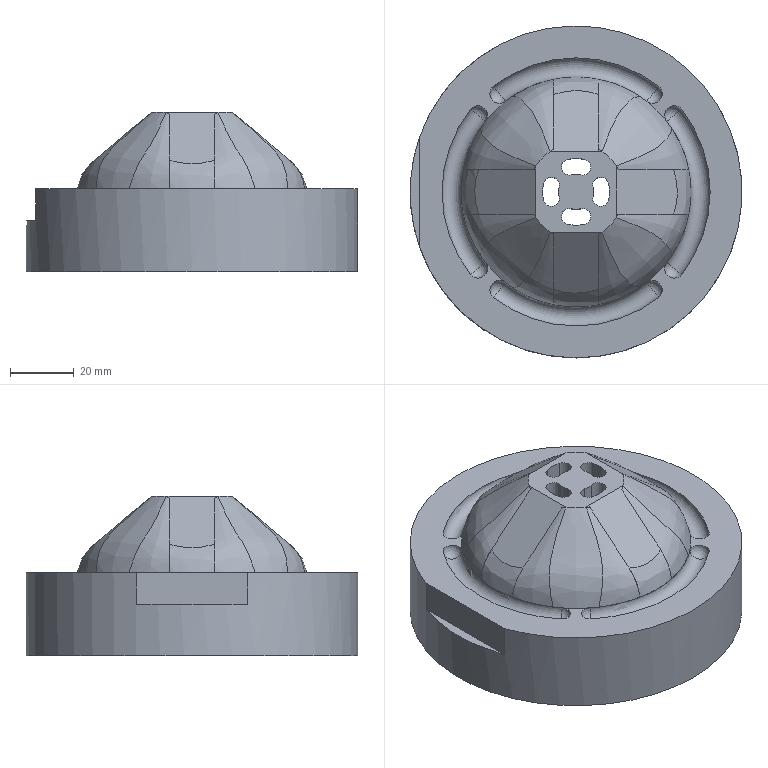NC program | NX | posted with a generic post | part box 104 x 104 x 49.86 mm
Lines 4139 to 5049 of 41131:
(ZLEVEL_PROFILE , TOOL : B12)
N8258 M6
N8260 G54
N8262 G17 G0 G90 X-5.745 Y-14.748 S3000 M3
N8264 G43 Z20. H0
N8266 Z0.2
N8268 G94 G1 X-6.948 Z0.168 F2000.
N8270 X-8.842 Y-14.619 Z0.119
N8272 X-9.264 Y-14.407 Z0.106
N8274 X-10.132 Y-13.832 Z0.079
N8276 X-12.11 Y-12.117 Z0.011
N8278 X-13.819 Y-10.134 Z-0.058
N8280 X-14.392 Y-9.264 Z-0.085
N8282 X-14.748 Y-8.085 Z-0.117
N8284 Y-1.181 Z-0.298
N8286 Y6.955 F2500.
N8288 X-14.7 Y6.986
N8290 X-14.632 Y8.788
N8292 X-14.619 Y8.842
N8294 G2 X-10.106 Y13.782 R13.681
N8296 G1 X-9.584 Y14.169
N8298 G2 X-8.085 Y14.748 R3.009
N8300 G1 X8.085
N8302 G2 X9.419 Y14.301 R2.214
N8304 G1 X10.506 Y13.48
N8306 G2 X14.182 Y9.513 R15.361
N8308 X14.748 Y8.085 R3.997
N8310 G1 Y-8.085
N8312 G2 X14.301 Y-9.419 R2.214
N8314 G1 X13.48 Y-10.506
N8316 G2 X9.513 Y-14.182 R15.361
N8318 X8.09 Y-14.748 R4.007
N8320 G1 X-6.948
N8322 X-8.842 Y-14.619
N8324 X-9.264 Y-14.407
N8326 G2 X-14.392 Y-9.264 R18.072
N8328 G1 X-14.748 Y-8.085
N8330 Y-1.181
N8332 X-15.113 Z-0.447
N8334 X-15.424 Z-0.597
N8336 Y-8.085
N8338 X-15.174 Y-9.264
N8340 G3 X-9.376 Y-15.111 R17.587
N8342 X-8.392 Y-15.39 R1.871
N8344 G1 X-6.983
N8346 X-6.953 Y-15.424
N8348 X8.09
N8350 X9.264 Y-15.174
N8352 G3 X15.062 Y-9.454 R17.608
N8354 X15.424 Y-8.194 R2.377
N8356 G1 Y8.087
N8358 X15.174 Y9.264
N8360 G3 X9.454 Y15.062 R17.608
N8362 X8.194 Y15.424 R2.377
N8364 G1 X-8.085
N8366 X-9.264 Y15.174
N8368 G3 X-14.097 Y10.803 R16.688
N8370 G1 X-14.907 Y9.713
N8372 G3 X-15.375 Y8.421 R2.263
N8374 G1 X-15.39 Y6.983
N8376 X-15.424 Y6.953
N8378 Y-1.181
N8380 X-15.696 Z-0.746
N8382 X-15.939 Z-0.895
N8384 Y6.951
N8386 X-15.855 Y8.85
N8388 X-15.733 Y9.264
N8390 G2 X-9.826 Y15.439 R17.411
N8392 X-8.088 Y15.939 R3.274
N8394 G1 X8.013
N8396 G2 X9.959 Y15.359 R3.557
N8398 X15.262 Y10.106 R18.618
N8400 X15.939 Y8.09 R3.89
N8402 G1 Y-8.013
N8404 G2 X15.359 Y-9.959 R3.557
N8406 X10.106 Y-15.262 R18.618
N8408 X8.09 Y-15.939 R3.891
N8410 G1 X-7.
N8412 X-8.85 Y-15.855
N8414 X-9.264 Y-15.733
N8416 G2 X-15.439 Y-9.826 R17.411
N8418 X-15.939 Y-8.088 R3.274
N8420 G1 Y-1.181
N8422 X-16.158 Z-1.044
N8424 X-16.359 Z-1.193
N8426 Y-8.1
N8428 G3 X-15.766 Y-10.106 R3.673
N8430 X-9.663 Y-16.001 R17.956
N8432 X-7. Y-16.359 R5.641
N8434 G1 X8.
N8436 G3 X10.106 Y-15.766 R3.809
N8438 X15.766 Y-10.106 R18.763
N8440 X16.359 Y-8.094 R3.673
N8442 G1 Y8.
N8444 G3 X15.766 Y10.106 R3.809
N8446 X10.106 Y15.766 R18.763
N8448 X8.094 Y16.359 R3.673
N8450 G1 X-8.16
N8452 G3 X-10.052 Y15.805 R3.507
N8454 X-15.159 Y11.001 R19.049
N8456 G1 X-15.583 Y10.419
N8458 G3 X-16.342 Y8.051 R3.95
N8460 G1 X-16.331 Y6.983
N8462 X-16.359 Y6.953
N8464 Y-1.181
N8466 X-16.544 Z-1.342
N8468 X-16.722 Z-1.491
N8470 Y8.301
N8472 G2 X-16.08 Y10.384 R3.7
N8474 X-15.159 Y11.651 R25.733
N8476 X-10.177 Y16.197 R19.698
N8478 X-8.377 Y16.722 R3.347
N8480 G1 X7.629
N8482 G2 X10.262 Y16.142 R3.863
N8484 X16.211 Y10.156 R19.742
N8486 X16.722 Y8.399 R3.271
N8488 G1 Y-7.629
N8490 G2 X16.142 Y-10.262 R3.863
N8492 X10.156 Y-16.211 R19.738
N8494 X8.399 Y-16.722 R3.271
N8496 G1 X-7.83
N8498 G2 X-10.187 Y-16.191 R3.553
N8500 X-16.21 Y-10.157 R19.734
N8502 X-16.722 Y-8.398 R3.277
N8504 G1 Y-1.181
N8506 X-17.078 Z-1.79
N8508 Y-7.086
N8510 X-17.079 Y-7.153
N8512 X-17.096 Y-7.579
N8514 X-17.11 Y-8.422
N8516 G3 X-16.695 Y-10.106 R4.099
N8518 X-10.106 Y-16.695 R20.371
N8520 X-7.089 Y-17.078 R5.61
N8522 G1 X7.086
N8524 X7.153 Y-17.079
N8526 X7.579 Y-17.096
N8528 X8.421 Y-17.11
N8530 G3 X10.106 Y-16.695 R4.115
N8532 X16.695 Y-10.106 R20.423
N8534 X17.078 Y-7.089 R5.61
N8536 G1 Y7.097
N8538 X17.08 Y7.136
N8540 X17.096 Y7.579
N8542 X17.11 Y8.421
N8544 G3 X16.695 Y10.106 R4.115
N8546 X10.106 Y16.695 R20.423
N8548 X7.089 Y17.078 R5.554
N8550 G1 X-7.097
N8552 X-7.171 Y17.079
N8554 X-7.579 Y17.096
N8556 X-8.422 Y17.11
N8558 G3 X-10.106 Y16.695 R4.099
N8560 X-16.418 Y10.586 R20.977
N8562 X-17.109 Y8.421 R4.089
N8564 G1 X-17.098 Y7.579
N8566 X-17.079 Y7.1
N8568 X-17.078 Y7.
N8570 Y-1.181
N8572 X-17.433 Z-2.088
N8574 Y6.8
N8576 X-17.493 Y8.05
N8578 G2 X-17.129 Y10.106 R4.7
N8580 X-10.245 Y17.044 R20.39
N8582 X-8.381 Y17.515 R3.25
N8584 G1 X-6.849 Y17.433
N8586 X6.876
N8588 X7.5 Y17.493
N8590 G2 X10.106 Y17.129 R5.65
N8592 X17.01 Y10.302 R20.395
N8594 X17.511 Y8.339 R3.419
N8596 G1 X17.433 Y6.815
N8598 Y-6.876
N8600 X17.488 Y-7.449
N8602 G2 X17.129 Y-10.106 R5.868
N8604 X10.312 Y-17.004 R20.387
N8606 X8.323 Y-17.511 R3.455
N8608 G1 X6.831 Y-17.433
N8610 X-6.876
N8612 X-7.449 Y-17.488
N8614 G2 X-10.106 Y-17.129 R5.868
N8616 X-17.04 Y-10.253 R20.382
N8618 X-17.514 Y-8.381 R3.268
N8620 G1 X-17.433 Y-6.831
N8622 Y-1.181
N8624 X-17.788 Z-2.386
N8626 Y-6.701
N8628 G3 X-17.553 Y-10.106 R7.601
N8630 X-10.106 Y-17.553 R20.25
N8632 X-7.824 Y-17.864 R5.669
N8634 G1 X-6.724 Y-17.788
N8636 X6.71
N8638 G3 X10.106 Y-17.553 R7.573
N8640 X17.553 Y-10.106 R20.25
N8642 X17.864 Y-7.824 R5.669
N8644 G1 X17.788 Y-6.724
N8646 Y6.71
N8648 G3 X17.553 Y10.106 R7.573
N8650 X10.106 Y17.553 R20.249
N8652 X7.824 Y17.864 R5.67
N8654 G1 X6.724 Y17.788
N8656 X-6.71
N8658 G3 X-10.106 Y17.553 R7.573
N8660 X-17.553 Y10.106 R20.25
N8662 X-17.864 Y7.824 R5.669
N8664 G1 X-17.788 Y6.724
N8666 Y-1.181
N8668 X-18.144 Z-2.684
N8670 Y6.672
N8672 X-18.224 Y7.539
N8674 G2 X-17.966 Y10.106 R6.747
N8676 X-17.02 Y11.696 R7.82
N8678 G1 X-16.563 Y12.29
N8680 G2 X-10.932 Y17.54 R23.494
N8682 X-9.06 Y18.194 R4.005
N8684 X-6.687 Y18.144 R11.148
N8686 G1 X6.688
N8688 X7.094 Y18.194
N8690 G2 X10.106 Y17.966 R7.677
N8692 X11.696 Y17.02 R7.82
N8694 G1 X12.29 Y16.563
N8696 G2 X17.54 Y10.932 R23.494
N8698 X18.194 Y9.06 R4.005
N8700 X18.144 Y6.687 R11.148
N8702 G1 Y-6.688
N8704 G2 X18.174 Y-9.264 R11.194
N8706 X17.53 Y-10.948 R3.848
N8708 G1 X17.237 Y-11.369
N8710 G2 X10.932 Y-17.541 R23.499
N8712 X9.06 Y-18.194 R4.005
N8714 X6.687 Y-18.144 R11.148
N8716 G1 X-6.672
N8718 G2 X-9.264 Y-18.174 R11.378
N8720 X-10.948 Y-17.53 R3.848
N8722 G1 X-11.369 Y-17.237
N8724 G2 X-17.499 Y-10.995 R23.503
N8726 X-18.235 Y-8.422 R4.381
N8728 G1 X-18.144 Y-6.671
N8730 Y-1.181
N8732 X-18.499 Z-2.983
N8734 Y-6.659
N8736 G3 X-18.553 Y-9.264 R10.995
N8738 X-17.972 Y-10.948 R3.879
N8740 X-12.522 Y-16.843 R24.466
N8742 G1 X-11.79 Y-17.394
N8744 G3 X-10.106 Y-18.374 R6.74
N8746 X-6.67 Y-18.499 R8.656
N8748 G1 X6.66
N8750 G3 X9.264 Y-18.553 R10.979
N8752 X10.948 Y-17.972 R3.879
N8754 X16.843 Y-12.522 R24.466
N8756 G1 X17.394 Y-11.79
N8758 G3 X18.374 Y-10.106 R6.74
N8760 X18.499 Y-6.671 R8.65
N8762 G1 Y6.66
N8764 G3 X18.553 Y9.264 R10.979
N8766 X17.972 Y10.948 R3.879
N8768 X12.522 Y16.843 R24.466
N8770 G1 X11.79 Y17.394
N8772 G3 X10.106 Y18.374 R6.74
N8774 X6.671 Y18.499 R8.579
N8776 G1 X-6.66
N8778 G3 X-9.264 Y18.553 R10.979
N8780 X-10.948 Y17.972 R3.879
N8782 X-16.843 Y12.522 R24.466
N8784 G1 X-17.394 Y11.79
N8786 G3 X-18.374 Y10.106 R6.74
N8788 X-18.499 Y6.67 R8.585
N8790 G1 Y-1.181
N8792 X-18.855 Z-3.281
N8794 Y6.67
N8796 G2 X-18.864 Y9.689 R10.28
N8798 X-18.186 Y11.313 R4.426
N8800 X-11.078 Y18.323 R25.6
N8802 X-9.543 Y18.89 R3.607
N8804 X-6.656 Y18.855 R10.588
N8806 G1 X6.67
N8808 G2 X9.689 Y18.864 R10.28
N8810 X11.313 Y18.186 R4.426
N8812 X18.323 Y11.078 R25.6
N8814 X18.89 Y9.543 R3.607
N8816 X18.855 Y6.656 R10.588
N8818 G1 Y-6.67
N8820 G2 X18.874 Y-9.625 R10.318
N8822 X18.339 Y-11.055 R3.488
N8824 X11.055 Y-18.339 R25.075
N8826 X9.566 Y-18.887 R3.543
N8828 X6.656 Y-18.855 R10.588
N8830 G1 X-6.67
N8832 G2 X-9.625 Y-18.874 R10.318
N8834 X-11.055 Y-18.339 R3.488
N8836 X-18.339 Y-11.055 R25.075
N8838 X-18.887 Y-9.566 R3.543
N8840 X-18.855 Y-6.656 R10.588
N8842 G1 Y-1.181
N8844 X-19.21 Z-3.579
N8846 Y-6.654
N8848 G3 X-18.83 Y-10.948 R7.396
N8850 X-10.948 Y-18.83 R25.355
N8852 X-6.671 Y-19.21 R7.369
N8854 G1 X6.654
N8856 G3 X10.948 Y-18.83 R7.396
N8858 X18.83 Y-10.948 R25.358
N8860 X19.21 Y-6.671 R7.369
N8862 G1 Y6.654
N8864 G3 X18.83 Y10.948 R7.396
N8866 X10.948 Y18.83 R25.362
N8868 X6.671 Y19.21 R7.369
N8870 G1 X-6.654
N8872 G3 X-10.948 Y18.83 R7.396
N8874 X-18.83 Y10.948 R25.358
N8876 X-19.21 Y6.671 R7.369
N8878 G1 Y-1.181
N8880 X-19.566 Z-3.877
N8882 Y6.671
N8884 G2 X-19.246 Y10.948 R8.171
N8886 X-10.948 Y19.246 R25.929
N8888 X-6.654 Y19.566 R8.196
N8890 G1 X6.671
N8892 G2 X10.948 Y19.246 R8.171
N8894 X19.246 Y10.948 R25.933
N8896 X19.566 Y6.654 R8.167
N8898 G1 Y-6.671
N8900 G2 X19.246 Y-10.948 R8.201
N8902 X10.948 Y-19.246 R25.929
N8904 X6.654 Y-19.566 R8.167
N8906 G1 X-6.671
N8908 G2 X-10.948 Y-19.246 R8.201
N8910 X-19.246 Y-10.948 R25.926
N8912 X-19.566 Y-6.654 R8.196
N8914 G1 Y-1.181
N8916 X-19.921 Z-4.176
N8918 Y-6.655
N8920 G3 X-19.913 Y-10.034 R10.045
N8922 X-19.259 Y-11.647 R4.103
N8924 X-14.317 Y-17.197 R28.93
N8926 G1 X-13.738 Y-17.685
N8928 G3 X-10.948 Y-19.646 R16.029
N8930 X-6.67 Y-19.921 R8.618
N8932 G1 X6.655
N8934 G3 X10.948 Y-19.646 R8.655
N8936 X17.197 Y-14.317 R25.014
N8938 X19.646 Y-10.948 R19.165
N8940 X19.921 Y-6.67 R8.618
N8942 G1 Y6.655
N8944 G3 X19.646 Y10.948 R8.655
N8946 X10.948 Y19.646 R25.479
N8948 X6.67 Y19.921 R8.604
N8950 G1 X-6.655
N8952 G3 X-10.948 Y19.646 R8.664
N8954 X-14.317 Y17.197 R19.16
N8956 X-19.646 Y10.948 R25.019
N8958 X-19.921 Y6.67 R8.604
N8960 G1 Y-1.181
N8962 X-20.277 Z-4.474
N8964 Y6.669
N8966 G2 X-20.04 Y10.948 R9.049
N8968 X-19.025 Y12.593 R8.93
N8970 G1 X-18.339 Y13.474
N8972 G2 X-11.886 Y19.52 R29.381
N8974 X-9.909 Y20.302 R4.767
N8976 X-6.657 Y20.277 R10.218
N8978 G1 X6.669
N8980 G2 X10.948 Y20.04 R9.049
N8982 X12.593 Y19.025 R8.93
N8984 G1 X13.474 Y18.339
N8986 G2 X19.545 Y11.849 R29.381
N8988 X20.291 Y9.976 R4.604
N8990 X20.277 Y6.657 R10.218
N8992 G1 Y-6.669
N8994 G2 X20.04 Y-10.948 R9.079
N8996 X19.025 Y-12.593 R8.93
N8998 G1 X18.339 Y-13.474
N9000 G2 X11.849 Y-19.545 R29.381
N9002 X9.977 Y-20.291 R4.604
N9004 X6.657 Y-20.277 R10.218
N9006 G1 X-6.669
N9008 G2 X-10.948 Y-20.04 R9.079
N9010 X-12.593 Y-19.025 R8.93
N9012 G1 X-13.474 Y-18.339
N9014 G2 X-19.52 Y-11.886 R29.381
N9016 X-20.302 Y-9.909 R4.767
N9018 X-20.277 Y-6.657 R10.218
N9020 G1 Y-1.181
N9022 X-20.632 Z-4.772
N9024 Y-6.664
N9026 G3 X-20.634 Y-10.106 R10.237
N9028 X-20.018 Y-11.79 R4.556
N9030 X-11.79 Y-20.018 R31.109
N9032 G1 X-10.948 Y-20.426
N9034 G3 X-6.668 Y-20.632 R9.475
N9036 G1 X6.664
N9038 G3 X10.106 Y-20.634 R10.237
N9040 X11.79 Y-20.018 R4.556
N9042 X20.018 Y-11.79 R31.109
N9044 G1 X20.426 Y-10.948
N9046 G3 X20.632 Y-6.668 R9.475
N9048 G1 Y6.664
N9050 G3 X20.634 Y10.106 R10.237
N9052 X20.018 Y11.79 R4.556
N9054 X11.79 Y20.018 R31.109
N9056 G1 X10.948 Y20.426
N9058 G3 X6.668 Y20.632 R9.475
N9060 G1 X-6.664
N9062 G3 X-10.106 Y20.634 R10.237
N9064 X-11.79 Y20.018 R4.556
N9066 X-20.018 Y11.79 R31.109
N9068 G1 X-20.426 Y10.948
N9070 G3 X-20.632 Y6.668 R9.475
N9072 G1 Y-1.181
N9074 X-20.988 Z-5.07
N9076 Y6.659
N9078 G2 X-20.993 Y10.109 R9.79
N9080 X-20.087 Y12.299 R5.507
N9082 X-11.79 Y20.435 R31.433
N9084 X-6.672 Y20.988 R8.061
N9086 G1 X6.659
N9088 G2 X10.109 Y20.993 R9.79
N9090 X12.299 Y20.087 R5.508
N9092 X20.435 Y11.79 R31.437
N9094 X20.988 Y6.672 R8.061
N9096 G1 Y-6.659
N9098 G2 X20.991 Y-10.122 R9.79
N9100 X20.091 Y-12.294 R5.482
N9102 X11.79 Y-20.435 R31.437
N9104 X6.672 Y-20.988 R8.061
N9106 G1 X-6.659
N9108 G2 X-10.122 Y-20.991 R9.79
N9110 X-12.294 Y-20.091 R5.481
N9112 X-20.435 Y-11.79 R31.433
N9114 X-20.988 Y-6.672 R8.061
N9116 G1 Y-1.181
N9118 X-21.343 Z-5.369
N9120 Y-6.675
N9122 G3 X-20.845 Y-11.79 R8.637
N9124 X-11.79 Y-20.844 R31.525
N9126 X-6.642 Y-21.343 R8.678
N9128 G1 X6.675
N9130 G3 X11.79 Y-20.845 R8.653
N9132 X20.844 Y-11.79 R31.525
N9134 X21.343 Y-6.642 R8.678
N9136 G1 Y6.675
N9138 G3 X20.845 Y11.79 R8.653
N9140 X11.79 Y20.845 R31.525
N9142 X6.642 Y21.343 R8.7
N9144 G1 X-6.675
N9146 G3 X-11.79 Y20.845 R8.637
N9148 X-20.845 Y11.79 R31.525
N9150 X-21.343 Y6.642 R8.683
N9152 G1 Y-1.181
N9154 X-21.698 Z-5.667
N9156 Y6.626
N9158 G2 X-21.245 Y11.79 R9.426
N9160 X-11.79 Y21.245 R31.431
N9162 X-6.678 Y21.698 R9.319
N9164 G1 X6.626
N9166 G2 X11.79 Y21.245 R9.422
N9168 X21.245 Y11.79 R31.434
N9170 X21.698 Y6.678 R9.311
N9172 G1 Y-6.626
N9174 G2 X21.245 Y-11.79 R9.449
N9176 X11.79 Y-21.245 R31.429
N9178 X6.678 Y-21.698 R9.311
N9180 G1 X-6.626
N9182 G2 X-11.79 Y-21.245 R9.449
N9184 X-21.245 Y-11.79 R31.426
N9186 X-21.698 Y-6.678 R9.319
N9188 G1 Y-1.181
N9190 X-22.054 Z-5.965
N9192 Y-6.679
N9194 G3 X-21.636 Y-11.79 R9.692
N9196 X-18.527 Y-15.928 R25.277
N9198 X-11.79 Y-21.635 R29.623
N9200 X-6.616 Y-22.054 R9.928
N9202 G1 X6.679
N9204 G3 X11.79 Y-21.636 R9.682
N9206 X15.928 Y-18.527 R25.277
N9208 X21.635 Y-11.79 R29.623
N9210 X22.054 Y-6.616 R9.928
N9212 G1 Y6.679
N9214 G3 X21.636 Y11.79 R9.682
N9216 X18.527 Y15.928 R25.277
N9218 X11.79 Y21.635 R29.623
N9220 X6.616 Y22.054 R9.913
N9222 G1 X-6.679
N9224 G3 X-11.79 Y21.636 R9.692
N9226 X-15.928 Y18.527 R25.277
N9228 X-21.635 Y11.79 R29.622
N9230 X-22.054 Y6.616 R9.919
N9232 G1 Y-1.181
N9234 X-22.409 Z-6.264
N9236 Y6.614
N9238 G2 X-21.896 Y12.04 R9.825
N9240 X-17.313 Y17.685 R28.581
N9242 X-12.04 Y21.896 R28.257
N9244 X-6.679 Y22.409 R9.514
N9246 G1 X6.614
N9248 G2 X12.04 Y21.896 R9.825
N9250 X17.685 Y17.313 R28.582
N9252 X21.896 Y12.04 R28.256
N9254 X22.409 Y6.679 R9.514
N9256 G1 Y-6.614
N9258 G2 X21.896 Y-12.04 R9.825
N9260 X17.313 Y-17.685 R28.582
N9262 X12.04 Y-21.896 R28.256
N9264 X6.679 Y-22.409 R9.514
N9266 G1 X-6.614
N9268 G2 X-12.04 Y-21.896 R9.825
N9270 X-17.685 Y-17.313 R28.582
N9272 X-21.896 Y-12.04 R28.256
N9274 X-22.409 Y-6.679 R9.514
N9276 G1 Y-1.181
N9278 X-22.765 Z-6.562
N9280 Y-6.68
N9282 G3 X-22.68 Y-10.779 R10.338
N9284 X-21.623 Y-13.145 R6.537
N9286 X-12.996 Y-21.725 R36.224
N9288 X-11.093 Y-22.599 R5.753
N9290 X-6.612 Y-22.765 R10.709
N9292 G1 X6.68
N9294 G3 X10.779 Y-22.68 R10.338
N9296 X13.145 Y-21.623 R6.537
N9298 X21.725 Y-12.996 R36.224
N9300 X22.599 Y-11.093 R5.753
N9302 X22.765 Y-6.612 R10.709
N9304 G1 Y6.68
N9306 G3 X22.68 Y10.779 R10.338
N9308 X21.623 Y13.145 R6.537
N9310 X12.996 Y21.725 R36.224
N9312 X11.093 Y22.599 R5.753
N9314 X6.612 Y22.765 R10.709
N9316 G1 X-6.68
N9318 G3 X-10.779 Y22.68 R10.338
N9320 X-13.145 Y21.623 R6.537
N9322 X-21.725 Y12.996 R36.224
N9324 X-22.599 Y11.093 R5.753
N9326 X-22.765 Y6.612 R10.709
N9328 G1 Y-1.181
N9330 X-23.12 Z-6.86
N9332 Y6.62
N9334 G2 X-22.39 Y12.632 R9.659
N9336 X-12.632 Y22.39 R36.686
N9338 X-6.693 Y23.12 R9.673
N9340 G1 X6.62
N9342 G2 X12.632 Y22.39 R9.659
N9344 X22.39 Y12.632 R36.686
N9346 X23.12 Y6.693 R9.602
N9348 G1 Y-6.62
N9350 G2 X22.39 Y-12.632 R9.755
N9352 X12.632 Y-22.39 R36.686
N9354 X6.693 Y-23.12 R9.602
N9356 G1 X-6.62
N9358 G2 X-12.632 Y-22.39 R9.755
N9360 X-22.39 Y-12.632 R36.686
N9362 X-23.12 Y-6.693 R9.673
N9364 G1 Y-1.181
N9366 X-23.476 Z-7.158
N9368 Y-6.705
N9370 G3 X-22.795 Y-12.632 R10.326
N9372 X-12.632 Y-22.795 R36.889
N9374 X-6.628 Y-23.476 R10.478
N9376 G1 X6.705
N9378 G3 X12.632 Y-22.795 R10.32
N9380 X22.795 Y-12.632 R36.889
N9382 X23.476 Y-6.628 R10.478
N9384 G1 Y6.705
N9386 G3 X22.795 Y12.632 R10.32
N9388 X12.632 Y22.795 R36.889
N9390 X6.628 Y23.476 R10.465
N9392 G1 X-6.705
N9394 G3 X-12.632 Y22.795 R10.326
N9396 X-22.795 Y12.632 R36.889
N9398 X-23.476 Y6.628 R10.465
N9400 G1 Y-1.181
N9402 X-23.831 Z-7.457
N9404 Y6.636
N9406 G2 X-23.187 Y12.632 R10.833
N9408 X-12.632 Y23.187 R36.538
N9410 X-6.708 Y23.831 R10.731
N9412 G1 X6.636
N9414 G2 X12.632 Y23.187 R10.833
N9416 X23.187 Y12.632 R36.537
N9418 X23.831 Y6.708 R10.726
N9420 G1 Y-6.636
N9422 G2 X23.187 Y-12.632 R10.855
N9424 X12.632 Y-23.187 R36.537
N9426 X6.708 Y-23.831 R10.726
N9428 G1 X-6.636
N9430 G2 X-12.632 Y-23.187 R10.855
N9432 X-23.187 Y-12.632 R36.538
N9434 X-23.831 Y-6.708 R10.731
N9436 G1 Y-1.181
N9438 X-24.187 Z-7.755
N9440 Y-6.702
N9442 G3 X-23.579 Y-12.632 R11.183
N9444 X-18.843 Y-18.527 R33.01
N9446 X-12.632 Y-23.578 R33.264
N9448 X-6.644 Y-24.187 R11.234
N9450 G1 X6.702
N9452 G3 X12.632 Y-23.579 R11.183
N9454 X18.527 Y-18.843 R33.009
N9456 X23.578 Y-12.632 R33.264
N9458 X24.187 Y-6.644 R11.234
N9460 G1 Y6.702
N9462 G3 X23.579 Y12.632 R11.183
N9464 X18.843 Y18.527 R33.01
N9466 X12.628 Y23.58 R33.059
N9468 X6.644 Y24.187 R11.235
N9470 G1 X-6.702
N9472 G3 X-12.632 Y23.579 R11.183
N9474 X-18.527 Y18.843 R33.01
N9476 X-23.58 Y12.628 R33.058
N9478 X-24.187 Y6.644 R11.235
N9480 G1 Y-1.181
N9482 X-24.542 Z-8.053
N9484 Y6.652
N9486 G2 X-24.193 Y11.937 R11.403
N9488 X-23.315 Y13.717 R6.308
N9490 X-13.497 Y23.465 R40.275
N9492 X-11.218 Y24.404 R5.68
N9494 G1 X-10.469 Y24.534
N9496 G2 X-6.688 Y24.542 R11.206
N9498 G1 X6.652
N9500 G2 X11.937 Y24.193 R11.403
N9502 X13.717 Y23.315 R6.308
N9504 X23.465 Y13.497 R40.275
N9506 X24.404 Y11.218 R5.68
N9508 G1 X24.534 Y10.469
N9510 G2 X24.542 Y6.688 R11.206
N9512 G1 Y-6.652
N9514 G2 X24.193 Y-11.937 R11.403
N9516 X23.315 Y-13.717 R6.308
N9518 X13.497 Y-23.465 R40.275
N9520 X11.218 Y-24.404 R5.68
N9522 G1 X10.469 Y-24.534
N9524 G2 X6.688 Y-24.542 R11.206
N9526 G1 X-6.652
N9528 G2 X-11.937 Y-24.193 R11.403
N9530 X-13.717 Y-23.315 R6.308
N9532 X-23.465 Y-13.497 R40.275
N9534 X-24.404 Y-11.218 R5.68
N9536 G1 X-24.534 Y-10.469
N9538 G2 X-24.542 Y-6.688 R11.206
N9540 G1 Y-1.181
N9542 X-24.898 Z-8.351
N9544 Y-6.682
N9546 G3 X-23.907 Y-13.474 R10.755
N9548 X-13.474 Y-23.906 R41.308
N9550 X-6.658 Y-24.898 R10.776
N9552 G1 X6.682
N9554 G3 X13.474 Y-23.907 R10.755
N9556 X23.906 Y-13.474 R41.308
N9558 X24.898 Y-6.658 R10.776
N9560 G1 Y6.682
N9562 G3 X23.907 Y13.474 R10.755
N9564 X13.474 Y23.906 R41.308
N9566 X6.658 Y24.898 R10.776
N9568 G1 X-6.682
N9570 G3 X-13.474 Y23.907 R10.755
N9572 X-23.906 Y13.474 R41.308
N9574 X-24.898 Y6.658 R10.776
N9576 G1 Y-1.181
N9578 X-25.253 Z-8.65
N9580 Y6.664
N9582 G2 X-24.316 Y13.474 R11.423
N9584 X-13.474 Y24.316 R41.702
N9586 X-6.677 Y25.253 R11.418
N9588 G1 X6.664
N9590 G2 X13.474 Y24.316 R11.429
N9592 X24.316 Y13.474 R41.702
N9594 X25.253 Y6.677 R11.418
N9596 G1 Y-6.664
N9598 G2 X24.316 Y-13.474 R11.423
N9600 X13.474 Y-24.316 R41.702
N9602 X6.677 Y-25.253 R11.418
N9604 G1 X-6.664
N9606 G2 X-13.474 Y-24.316 R11.423
N9608 X-24.316 Y-13.474 R41.702
N9610 X-25.253 Y-6.677 R11.418
N9612 G1 Y-1.181
N9614 X-25.609 Z-8.948
N9616 Y-6.677
N9618 G3 X-24.712 Y-13.474 R11.888
N9620 X-13.474 Y-24.712 R41.23
N9622 X-6.664 Y-25.609 R11.92
N9624 G1 X6.677
N9626 G3 X13.474 Y-24.712 R11.888
N9628 X24.712 Y-13.474 R41.233
N9630 X25.609 Y-6.664 R11.92
N9632 G1 Y6.677
N9634 G3 X24.712 Y13.474 R11.888
N9636 X13.474 Y24.712 R41.235
N9638 X6.664 Y25.609 R11.923
N9640 G1 X-6.677
N9642 G3 X-13.474 Y24.712 R11.888
N9644 X-24.712 Y13.474 R41.23
N9646 X-25.609 Y6.664 R11.92
N9648 G1 Y-1.181
N9650 X-25.964 Z-9.246
N9652 Y6.664
N9654 G2 X-25.103 Y13.474 R12.416
N9656 X-13.474 Y25.103 R40.73
N9658 X-6.677 Y25.964 R12.339
N9660 G1 X6.664
N9662 G2 X13.474 Y25.103 R12.416
N9664 X25.103 Y13.474 R40.729
N9666 X25.964 Y6.677 R12.339
N9668 G1 Y-6.664
N9670 G2 X24.86 Y-13.909 R11.861
N9672 X13.474 Y-25.103 R42.052
N9674 X6.677 Y-25.964 R12.339
N9676 G1 X-6.664
N9678 G2 X-13.909 Y-24.86 R11.861
N9680 X-25.103 Y-13.474 R42.052
N9682 X-25.964 Y-6.677 R12.339
N9684 G1 Y-1.181
N9686 X-26.319 Z-9.544
N9688 Y-6.686
N9690 G3 X-25.264 Y-13.877 R12.126
N9692 X-13.891 Y-25.264 R42.6
N9694 X-6.664 Y-26.319 R12.268
N9696 G1 X6.686
N9698 G3 X13.745 Y-25.358 R12.537
N9700 X25.264 Y-13.891 R42.707
N9702 X26.319 Y-6.664 R12.268
N9704 G1 Y6.686
N9706 G3 X25.358 Y13.745 R12.537
N9708 X13.745 Y25.358 R42.576
N9710 X6.664 Y26.319 R12.619
N9712 G1 X-6.686
N9714 G3 X-13.877 Y25.264 R12.125
N9716 X-25.358 Y13.745 R42.455
N9718 X-26.319 Y6.664 R12.619
N9720 G1 Y-1.181
N9722 X-26.675 Z-9.843
N9724 Y6.664
N9726 G2 X-25.662 Y13.91 R12.894
N9728 X-14.317 Y25.412 R43.994
N9730 X-6.701 Y26.675 R12.011
N9732 G1 X6.664
N9734 G2 X13.91 Y25.662 R12.894
N9736 X25.663 Y13.91 R43.273
N9738 X26.675 Y6.701 R12.786
N9740 G1 Y-6.664
N9742 G2 X25.412 Y-14.317 R12.053
N9744 X13.91 Y-25.663 R43.992
N9746 X6.701 Y-26.675 R12.786
N9748 G1 X-6.664
N9750 G2 X-14.317 Y-25.412 R12.053
N9752 X-25.412 Y-14.317 R44.981
N9754 X-26.675 Y-6.701 R12.011
N9756 G1 Y-1.181
N9758 X-27.03 Z-10.141
N9760 Y-6.716
N9762 G3 X-25.823 Y-14.317 R12.665
N9764 X-14.317 Y-25.823 R45.122
N9766 X-6.664 Y-27.03 R12.776
N9768 G1 X6.716
N9770 G3 X14.075 Y-25.968 R13.018
N9772 X25.823 Y-14.317 R44.542
N9774 X27.03 Y-6.664 R12.776
N9776 G1 Y6.716
N9778 G3 X25.968 Y14.075 R13.018
N9780 X14.075 Y25.967 R43.973
N9782 X6.664 Y27.03 R13.145
N9784 G1 X-6.716
N9786 G3 X-14.317 Y25.823 R12.665
N9788 X-25.967 Y14.075 R44.53
N9790 X-27.03 Y6.664 R13.145
N9792 G1 Y-1.181
N9794 X-27.386 Z-10.439
N9796 Y6.667
N9798 G2 X-26.227 Y14.317 R13.313
N9800 X-14.317 Y26.228 R45.036
N9802 X-6.739 Y27.386 R13.164
N9804 G1 X6.667
N9806 G2 X14.317 Y26.227 R13.313
N9808 X26.228 Y14.317 R45.037
N9810 X27.386 Y6.739 R13.164
N9812 G1 Y-6.667
N9814 G2 X26.227 Y-14.317 R13.313
N9816 X14.317 Y-26.228 R45.037
N9818 X6.739 Y-27.386 R13.164
N9820 G1 X-6.667
N9822 G2 X-14.317 Y-26.227 R13.313
N9824 X-26.228 Y-14.317 R45.036
N9826 X-27.386 Y-6.739 R13.164
N9828 G1 Y-1.181
N9830 X-27.741 Z-10.738
N9832 Y-6.76
N9834 G3 X-26.385 Y-14.727 R13.129
N9836 X-14.317 Y-26.618 R45.439
N9838 X-6.67 Y-27.741 R13.714
N9840 G1 X6.76
N9842 G3 X14.317 Y-26.618 R13.542
N9844 X26.618 Y-14.317 R44.138
N9846 X27.741 Y-6.67 R13.714
N9848 G1 Y6.76
N9850 G3 X26.618 Y14.317 R13.542
N9852 X14.317 Y26.618 R44.138
N9854 X6.67 Y27.741 R13.714
N9856 G1 X-6.76
N9858 G3 X-14.727 Y26.385 R13.129
N9860 X-26.618 Y14.317 R45.439
N9862 X-27.741 Y6.67 R13.714
N9864 G1 Y-1.181
N9866 X-28.097 Z-11.036
N9868 Y6.684
N9870 G2 X-26.955 Y14.429 R14.107
N9872 X-14.905 Y26.681 R45.484
N9874 X-6.763 Y28.097 R13.432
N9876 G1 X6.684
N9878 G2 X14.429 Y26.955 R14.107
N9880 X26.955 Y14.429 R44.335
N9882 X28.097 Y6.763 R13.939
N9884 G1 Y-6.684
N9886 G2 X26.949 Y-14.424 R13.99
N9888 X14.429 Y-26.955 R43.539
N9890 X6.763 Y-28.097 R13.939
N9892 G1 X-6.684
N9894 G2 X-14.424 Y-26.949 R13.99
N9896 X-26.681 Y-14.905 R44.033
N9898 X-28.097 Y-6.763 R13.432
N9900 G1 Y-1.181
N9902 X-28.452 Z-11.334
N9904 Y-6.763
N9906 G3 X-26.949 Y-15.126 R13.651
N9908 X-15.12 Y-26.949 R47.206
N9910 X-6.699 Y-28.452 R13.734
N9912 G1 X6.763
N9914 G3 X15.122 Y-26.949 R13.366
N9916 X26.949 Y-15.12 R47.136
N9918 X28.452 Y-6.699 R13.734
N9920 G1 Y6.763
N9922 G3 X27.264 Y14.59 R14.259
N9924 X14.59 Y27.264 R44.456
N9926 X6.699 Y28.452 R14.413
N9928 G1 X-6.763
N9930 G3 X-15.126 Y26.949 R13.651
N9932 X-26.949 Y15.121 R47.222
N9934 X-28.452 Y6.699 R13.409
N9936 G1 Y-1.181
N9938 X-28.808 Z-11.632
N9940 Y6.716
N9942 G2 X-27.339 Y15.159 R14.249
N9944 X-15.159 Y27.34 R46.988
N9946 X-6.762 Y28.808 R14.172
N9948 G1 X6.716
N9950 G2 X15.159 Y27.339 R14.249
N9952 X27.34 Y15.159 R46.988
N9954 X28.808 Y6.762 R14.167
N9956 G1 Y-6.716
N9958 G2 X27.339 Y-15.159 R14.254
N9960 X15.159 Y-27.34 R46.988
N9962 X6.762 Y-28.808 R14.167
N9964 G1 X-6.716
N9966 G2 X-15.159 Y-27.339 R14.254
N9968 X-27.34 Y-15.159 R46.988
N9970 X-28.808 Y-6.762 R14.172
N9972 G1 Y-1.181
N9974 X-29.163 Z-11.931
N9976 Y-6.762
N9978 G3 X-27.753 Y-15.159 R14.817
N9980 X-15.159 Y-27.753 R46.495
N9982 X-6.736 Y-29.163 R14.863
N9984 G1 X6.762
N9986 G3 X15.159 Y-27.753 R14.817
N9988 X27.753 Y-15.159 R46.495
N9990 X29.163 Y-6.736 R14.863
N9992 G1 Y6.762
N9994 G3 X27.753 Y15.159 R14.817
N9996 X15.159 Y27.753 R46.495
N9998 X6.736 Y29.163 R14.863
N10000 G1 X-6.762
N10002 G3 X-15.159 Y27.753 R14.817
N10004 X-27.753 Y15.159 R46.495
N10006 X-29.163 Y6.736 R14.863
N10008 G1 Y-1.181
N10010 X-29.519 Z-12.229
N10012 Y6.759
N10014 G2 X-28.147 Y15.159 R15.266
N10016 X-15.159 Y28.148 R44.746
N10018 X-6.765 Y29.519 R15.261
N10020 G1 X6.759
N10022 G2 X15.159 Y28.147 R15.266
N10024 X28.148 Y15.159 R44.746
N10026 X29.519 Y6.765 R15.261
N10028 G1 Y-6.759
N10030 G2 X28.147 Y-15.159 R15.266
N10032 X15.159 Y-28.148 R44.746
N10034 X6.765 Y-29.519 R15.261
N10036 G1 X-6.759
N10038 G2 X-15.159 Y-28.147 R15.266
N10040 X-28.148 Y-15.159 R44.746
N10042 X-29.519 Y-6.765 R15.261
N10044 G1 Y-1.181
N10046 X-29.874 Z-12.527
N10048 Y-6.79
N10050 G3 X-28.054 Y-16.001 R14.709
N10052 X-16.001 Y-28.054 R47.067
N10054 X-6.781 Y-29.874 R14.712
N10056 G1 X6.79
N10058 G3 X16.001 Y-28.054 R14.709
N10060 X28.054 Y-16.001 R47.067
N10062 X29.874 Y-6.781 R14.712
N10064 G1 Y6.79
N10066 G3 X28.054 Y16.001 R14.709
N10068 X16.001 Y28.054 R47.067
N10070 X6.781 Y29.874 R14.712
N10072 G1 X-6.79